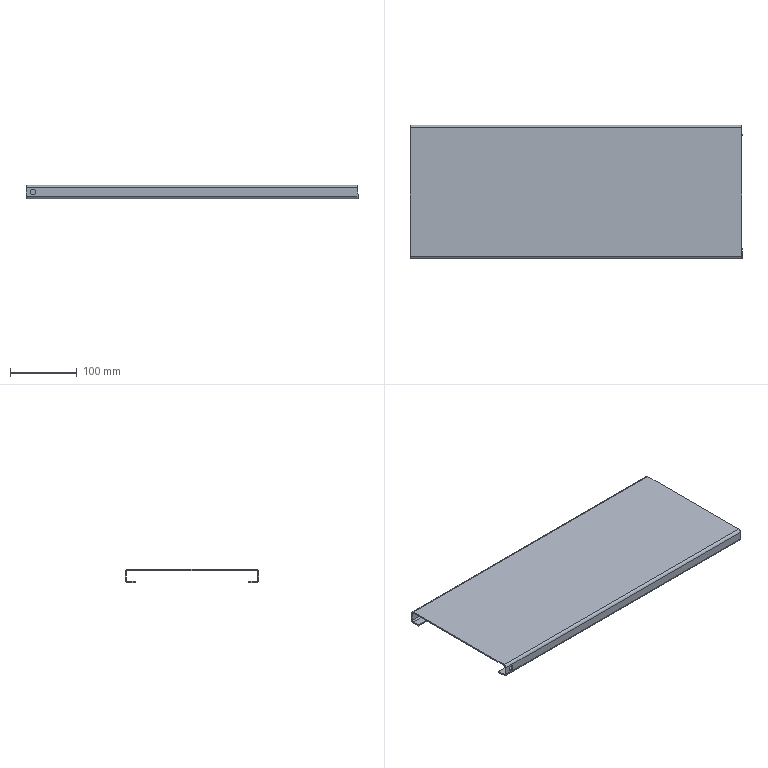Part | SolidWorks | features EdgeFlange 4, Extrusion 1, FlatPattern 1, ICE 1, SheetMetal 1, SolidToSheetMetal 1 | 1 solid | 40 faces | box 496 x 200 x 20 mm | volume 254694 mm3 | plane 30 | cylinder 10 | commonest cylinder face diameters 8 x6 4 x4
STEP:
#1=CARTESIAN_POINT('',(-237.5,-98.,-5.));
#2=VERTEX_POINT('',#1);
#3=CARTESIAN_POINT('',(-237.5,-98.,-13.));
#4=VERTEX_POINT('',#3);
#5=CARTESIAN_POINT('',(-237.5,-98.,-9.));
#6=DIRECTION('',(0.,-1.,0.));
#7=DIRECTION('',(0.,0.,-1.));
#8=AXIS2_PLACEMENT_3D('',#5,#6,#7);
#9=CIRCLE('',#8,4.);
#10=EDGE_CURVE('',#2,#4,#9,.T.);
#11=ORIENTED_EDGE('',*,*,#10,.F.);
#12=CARTESIAN_POINT('',(-237.5,-100.,-5.));
#13=VERTEX_POINT('',#12);
#14=CARTESIAN_POINT('',(-237.5,-98.,-5.));
#15=DIRECTION('',(0.,-1.,0.));
#16=VECTOR('',#15,1000.);
#17=LINE('',#14,#16);
#18=EDGE_CURVE('',#2,#13,#17,.T.);
#19=ORIENTED_EDGE('',*,*,#18,.T.);
#20=CARTESIAN_POINT('',(-237.5,-100.,-13.));
#21=VERTEX_POINT('',#20);
#22=CARTESIAN_POINT('',(-237.5,-100.,-9.));
#23=DIRECTION('',(0.,-1.,0.));
#24=DIRECTION('',(0.,0.,-1.));
#25=AXIS2_PLACEMENT_3D('',#22,#23,#24);
#26=CIRCLE('',#25,4.);
#27=EDGE_CURVE('',#13,#21,#26,.T.);
#28=ORIENTED_EDGE('',*,*,#27,.T.);
#29=CARTESIAN_POINT('',(-237.5,-98.,-13.));
#30=DIRECTION('',(0.,-1.,0.));
#31=VECTOR('',#30,1000.);
#32=LINE('',#29,#31);
#33=EDGE_CURVE('',#4,#21,#32,.T.);
#34=ORIENTED_EDGE('',*,*,#33,.F.);
#35=EDGE_LOOP('',(#11,#19,#28,#34));
#36=FACE_OUTER_BOUND('',#35,.T.);
#37=CARTESIAN_POINT('',(-237.5,-98.,-9.));
#38=DIRECTION('',(0.,-1.,0.));
#39=DIRECTION('',(0.,0.,-1.));
#40=AXIS2_PLACEMENT_3D('',#37,#38,#39);
#41=CYLINDRICAL_SURFACE('',#40,4.);
#42=ADVANCED_FACE('',(#36),#41,.F.);
#43=CARTESIAN_POINT('',(-248.,-98.,-15.));
#44=VERTEX_POINT('',#43);
#45=CARTESIAN_POINT('',(-248.,-98.,-3.));
#46=VERTEX_POINT('',#45);
#47=CARTESIAN_POINT('',(-248.,-98.,-1.));
#48=DIRECTION('',(0.,0.,1.));
#49=VECTOR('',#48,1000.);
#50=LINE('',#47,#49);
#51=EDGE_CURVE('',#44,#46,#50,.T.);
#52=ORIENTED_EDGE('',*,*,#51,.F.);
#53=CARTESIAN_POINT('',(-248.,-100.,-15.));
#54=VERTEX_POINT('',#53);
#55=CARTESIAN_POINT('',(-248.,-98.,-15.));
#56=DIRECTION('',(0.,-1.,0.));
#57=VECTOR('',#56,1000.);
#58=LINE('',#55,#57);
#59=EDGE_CURVE('',#44,#54,#58,.T.);
#60=ORIENTED_EDGE('',*,*,#59,.T.);
#61=CARTESIAN_POINT('',(-248.,-100.,-3.));
#62=VERTEX_POINT('',#61);
#63=CARTESIAN_POINT('',(-248.,-100.,-1.));
#64=DIRECTION('',(0.,0.,1.));
#65=VECTOR('',#64,1000.);
#66=LINE('',#63,#65);
#67=EDGE_CURVE('',#54,#62,#66,.T.);
#68=ORIENTED_EDGE('',*,*,#67,.T.);
#69=CARTESIAN_POINT('',(-248.,-98.,-3.));
#70=DIRECTION('',(0.,-1.,0.));
#71=VECTOR('',#70,1000.);
#72=LINE('',#69,#71);
#73=EDGE_CURVE('',#46,#62,#72,.T.);
#74=ORIENTED_EDGE('',*,*,#73,.F.);
#75=EDGE_LOOP('',(#52,#60,#68,#74));
#76=FACE_OUTER_BOUND('',#75,.T.);
#77=CARTESIAN_POINT('',(-248.,-100.,-1.));
#78=DIRECTION('',(-1.,0.,0.));
#79=DIRECTION('',(0.,0.,1.));
#80=AXIS2_PLACEMENT_3D('',#77,#78,#79);
#81=PLANE('',#80);
#82=ADVANCED_FACE('',(#76),#81,.T.);
#83=CARTESIAN_POINT('',(-237.5,-100.,-9.));
#84=DIRECTION('',(0.,-1.,0.));
#85=DIRECTION('',(0.,0.,-1.));
#86=AXIS2_PLACEMENT_3D('',#83,#84,#85);
#87=CIRCLE('',#86,4.);
#88=EDGE_CURVE('',#21,#13,#87,.T.);
#89=ORIENTED_EDGE('',*,*,#88,.F.);
#90=ORIENTED_EDGE('',*,*,#27,.F.);
#91=EDGE_LOOP('',(#89,#90));
#92=FACE_BOUND('',#91,.T.);
#93=ORIENTED_EDGE('',*,*,#67,.F.);
#94=CARTESIAN_POINT('',(248.,-100.,-15.));
#95=VERTEX_POINT('',#94);
#96=CARTESIAN_POINT('',(-248.,-100.,-15.));
#97=DIRECTION('',(1.,0.,0.));
#98=VECTOR('',#97,1000.);
#99=LINE('',#96,#98);
#100=EDGE_CURVE('',#54,#95,#99,.T.);
#101=ORIENTED_EDGE('',*,*,#100,.T.);
#102=CARTESIAN_POINT('',(248.,-100.,-3.));
#103=VERTEX_POINT('',#102);
#104=CARTESIAN_POINT('',(248.,-100.,-19.));
#105=DIRECTION('',(0.,0.,-1.));
#106=VECTOR('',#105,1000.);
#107=LINE('',#104,#106);
#108=EDGE_CURVE('',#103,#95,#107,.T.);
#109=ORIENTED_EDGE('',*,*,#108,.F.);
#110=CARTESIAN_POINT('',(-248.,-100.,-3.));
#111=DIRECTION('',(-1.,0.,0.));
#112=VECTOR('',#111,1000.);
#113=LINE('',#110,#112);
#114=EDGE_CURVE('',#103,#62,#113,.T.);
#115=ORIENTED_EDGE('',*,*,#114,.T.);
#116=EDGE_LOOP('',(#93,#101,#109,#115));
#117=FACE_OUTER_BOUND('',#116,.T.);
#118=CARTESIAN_POINT('',(-248.,-100.,-1.));
#119=DIRECTION('',(0.,-1.,0.));
#120=DIRECTION('',(0.,0.,-1.));
#121=AXIS2_PLACEMENT_3D('',#118,#119,#120);
#122=PLANE('',#121);
#123=ADVANCED_FACE('',(#92,#117),#122,.T.);
#124=CARTESIAN_POINT('',(-237.5,-98.,-9.));
#125=DIRECTION('',(0.,-1.,0.));
#126=DIRECTION('',(0.,0.,-1.));
#127=AXIS2_PLACEMENT_3D('',#124,#125,#126);
#128=CIRCLE('',#127,4.);
#129=EDGE_CURVE('',#4,#2,#128,.T.);
#130=ORIENTED_EDGE('',*,*,#129,.T.);
#131=ORIENTED_EDGE('',*,*,#10,.T.);
#132=EDGE_LOOP('',(#130,#131));
#133=FACE_BOUND('',#132,.T.);
#134=CARTESIAN_POINT('',(248.,-98.,-15.));
#135=VERTEX_POINT('',#134);
#136=CARTESIAN_POINT('',(-248.,-98.,-15.));
#137=DIRECTION('',(1.,0.,0.));
#138=VECTOR('',#137,1000.);
#139=LINE('',#136,#138);
#140=EDGE_CURVE('',#44,#135,#139,.T.);
#141=ORIENTED_EDGE('',*,*,#140,.F.);
#142=ORIENTED_EDGE('',*,*,#51,.T.);
#143=CARTESIAN_POINT('',(248.,-98.,-3.));
#144=VERTEX_POINT('',#143);
#145=CARTESIAN_POINT('',(248.,-98.,-3.));
#146=DIRECTION('',(-1.,0.,0.));
#147=VECTOR('',#146,1000.);
#148=LINE('',#145,#147);
#149=EDGE_CURVE('',#144,#46,#148,.T.);
#150=ORIENTED_EDGE('',*,*,#149,.F.);
#151=CARTESIAN_POINT('',(248.,-98.,-1.));
#152=DIRECTION('',(0.,0.,-1.));
#153=VECTOR('',#152,1000.);
#154=LINE('',#151,#153);
#155=EDGE_CURVE('',#144,#135,#154,.T.);
#156=ORIENTED_EDGE('',*,*,#155,.T.);
#157=EDGE_LOOP('',(#141,#142,#150,#156));
#158=FACE_OUTER_BOUND('',#157,.T.);
#159=CARTESIAN_POINT('',(-248.,-98.,-1.));
#160=DIRECTION('',(0.,-1.,0.));
#161=DIRECTION('',(0.,0.,-1.));
#162=AXIS2_PLACEMENT_3D('',#159,#160,#161);
#163=PLANE('',#162);
#164=ADVANCED_FACE('',(#133,#158),#163,.F.);
#165=CARTESIAN_POINT('',(-248.,96.,1.));
#166=VERTEX_POINT('',#165);
#167=CARTESIAN_POINT('',(-248.,-96.,1.));
#168=VERTEX_POINT('',#167);
#169=CARTESIAN_POINT('',(-248.,100.,1.));
#170=DIRECTION('',(0.,-1.,0.));
#171=VECTOR('',#170,1000.);
#172=LINE('',#169,#171);
#173=EDGE_CURVE('',#166,#168,#172,.T.);
#174=ORIENTED_EDGE('',*,*,#173,.T.);
#175=CARTESIAN_POINT('',(248.,-96.,1.));
#176=VERTEX_POINT('',#175);
#177=CARTESIAN_POINT('',(-248.,-96.,1.));
#178=DIRECTION('',(1.,0.,0.));
#179=VECTOR('',#178,1000.);
#180=LINE('',#177,#179);
#181=EDGE_CURVE('',#168,#176,#180,.T.);
#182=ORIENTED_EDGE('',*,*,#181,.T.);
#183=CARTESIAN_POINT('',(248.,96.,1.));
#184=VERTEX_POINT('',#183);
#185=CARTESIAN_POINT('',(248.,100.,1.));
#186=DIRECTION('',(0.,1.,0.));
#187=VECTOR('',#186,1000.);
#188=LINE('',#185,#187);
#189=EDGE_CURVE('',#176,#184,#188,.T.);
#190=ORIENTED_EDGE('',*,*,#189,.T.);
#191=CARTESIAN_POINT('',(248.,96.,1.));
#192=DIRECTION('',(-1.,0.,0.));
#193=VECTOR('',#192,1000.);
#194=LINE('',#191,#193);
#195=EDGE_CURVE('',#184,#166,#194,.T.);
#196=ORIENTED_EDGE('',*,*,#195,.T.);
#197=EDGE_LOOP('',(#174,#182,#190,#196));
#198=FACE_OUTER_BOUND('',#197,.T.);
#199=CARTESIAN_POINT('',(248.,-100.,1.));
#200=DIRECTION('',(0.,0.,1.));
#201=DIRECTION('',(1.,0.,0.));
#202=AXIS2_PLACEMENT_3D('',#199,#200,#201);
#203=PLANE('',#202);
#204=ADVANCED_FACE('',(#198),#203,.T.);
#205=CARTESIAN_POINT('',(-248.,-96.,-1.));
#206=VERTEX_POINT('',#205);
#207=CARTESIAN_POINT('',(248.,-96.,-1.));
#208=VERTEX_POINT('',#207);
#209=CARTESIAN_POINT('',(-248.,-96.,-1.));
#210=DIRECTION('',(1.,0.,0.));
#211=VECTOR('',#210,1000.);
#212=LINE('',#209,#211);
#213=EDGE_CURVE('',#206,#208,#212,.T.);
#214=ORIENTED_EDGE('',*,*,#213,.F.);
#215=CARTESIAN_POINT('',(-248.,96.,-1.));
#216=VERTEX_POINT('',#215);
#217=CARTESIAN_POINT('',(-248.,-100.,-1.));
#218=DIRECTION('',(0.,-1.,0.));
#219=VECTOR('',#218,1000.);
#220=LINE('',#217,#219);
#221=EDGE_CURVE('',#216,#206,#220,.T.);
#222=ORIENTED_EDGE('',*,*,#221,.F.);
#223=CARTESIAN_POINT('',(248.,96.,-1.));
#224=VERTEX_POINT('',#223);
#225=CARTESIAN_POINT('',(248.,96.,-1.));
#226=DIRECTION('',(-1.,0.,0.));
#227=VECTOR('',#226,1000.);
#228=LINE('',#225,#227);
#229=EDGE_CURVE('',#224,#216,#228,.T.);
#230=ORIENTED_EDGE('',*,*,#229,.F.);
#231=CARTESIAN_POINT('',(248.,-100.,-1.));
#232=DIRECTION('',(0.,1.,0.));
#233=VECTOR('',#232,1000.);
#234=LINE('',#231,#233);
#235=EDGE_CURVE('',#208,#224,#234,.T.);
#236=ORIENTED_EDGE('',*,*,#235,.F.);
#237=EDGE_LOOP('',(#214,#222,#230,#236));
#238=FACE_OUTER_BOUND('',#237,.T.);
#239=CARTESIAN_POINT('',(248.,-100.,-1.));
#240=DIRECTION('',(0.,0.,1.));
#241=DIRECTION('',(1.,0.,0.));
#242=AXIS2_PLACEMENT_3D('',#239,#240,#241);
#243=PLANE('',#242);
#244=ADVANCED_FACE('',(#238),#243,.F.);
#245=ORIENTED_EDGE('',*,*,#221,.T.);
#246=CARTESIAN_POINT('',(-248.,-96.,-1.));
#247=DIRECTION('',(0.,0.,1.));
#248=VECTOR('',#247,1000.);
#249=LINE('',#246,#248);
#250=EDGE_CURVE('',#206,#168,#249,.T.);
#251=ORIENTED_EDGE('',*,*,#250,.T.);
#252=ORIENTED_EDGE('',*,*,#173,.F.);
#253=CARTESIAN_POINT('',(-248.,96.,-1.));
#254=DIRECTION('',(0.,0.,1.));
#255=VECTOR('',#254,1000.);
#256=LINE('',#253,#255);
#257=EDGE_CURVE('',#216,#166,#256,.T.);
#258=ORIENTED_EDGE('',*,*,#257,.F.);
#259=EDGE_LOOP('',(#245,#251,#252,#258));
#260=FACE_OUTER_BOUND('',#259,.T.);
#261=CARTESIAN_POINT('',(-248.,100.,1.));
#262=DIRECTION('',(-1.,0.,0.));
#263=DIRECTION('',(0.,-1.,0.));
#264=AXIS2_PLACEMENT_3D('',#261,#262,#263);
#265=PLANE('',#264);
#266=ADVANCED_FACE('',(#260),#265,.T.);
#267=CARTESIAN_POINT('',(248.,98.,-15.));
#268=VERTEX_POINT('',#267);
#269=CARTESIAN_POINT('',(248.,98.,-3.));
#270=VERTEX_POINT('',#269);
#271=CARTESIAN_POINT('',(248.,98.,-1.));
#272=DIRECTION('',(0.,0.,1.));
#273=VECTOR('',#272,1000.);
#274=LINE('',#271,#273);
#275=EDGE_CURVE('',#268,#270,#274,.T.);
#276=ORIENTED_EDGE('',*,*,#275,.F.);
#277=CARTESIAN_POINT('',(248.,100.,-15.));
#278=VERTEX_POINT('',#277);
#279=CARTESIAN_POINT('',(248.,98.,-15.));
#280=DIRECTION('',(0.,1.,0.));
#281=VECTOR('',#280,1000.);
#282=LINE('',#279,#281);
#283=EDGE_CURVE('',#268,#278,#282,.T.);
#284=ORIENTED_EDGE('',*,*,#283,.T.);
#285=CARTESIAN_POINT('',(248.,100.,-3.));
#286=VERTEX_POINT('',#285);
#287=CARTESIAN_POINT('',(248.,100.,-1.));
#288=DIRECTION('',(0.,0.,1.));
#289=VECTOR('',#288,1000.);
#290=LINE('',#287,#289);
#291=EDGE_CURVE('',#278,#286,#290,.T.);
#292=ORIENTED_EDGE('',*,*,#291,.T.);
#293=CARTESIAN_POINT('',(248.,98.,-3.));
#294=DIRECTION('',(0.,1.,0.));
#295=VECTOR('',#294,1000.);
#296=LINE('',#293,#295);
#297=EDGE_CURVE('',#270,#286,#296,.T.);
#298=ORIENTED_EDGE('',*,*,#297,.F.);
#299=EDGE_LOOP('',(#276,#284,#292,#298));
#300=FACE_OUTER_BOUND('',#299,.T.);
#301=CARTESIAN_POINT('',(248.,100.,-1.));
#302=DIRECTION('',(1.,0.,0.));
#303=DIRECTION('',(0.,0.,-1.));
#304=AXIS2_PLACEMENT_3D('',#301,#302,#303);
#305=PLANE('',#304);
#306=ADVANCED_FACE('',(#300),#305,.T.);
#307=ORIENTED_EDGE('',*,*,#291,.F.);
#308=CARTESIAN_POINT('',(-248.,100.,-15.));
#309=VERTEX_POINT('',#308);
#310=CARTESIAN_POINT('',(248.,100.,-15.));
#311=DIRECTION('',(-1.,0.,0.));
#312=VECTOR('',#311,1000.);
#313=LINE('',#310,#312);
#314=EDGE_CURVE('',#278,#309,#313,.T.);
#315=ORIENTED_EDGE('',*,*,#314,.T.);
#316=CARTESIAN_POINT('',(-248.,100.,-3.));
#317=VERTEX_POINT('',#316);
#318=CARTESIAN_POINT('',(-248.,100.,-19.));
#319=DIRECTION('',(0.,0.,-1.));
#320=VECTOR('',#319,1000.);
#321=LINE('',#318,#320);
#322=EDGE_CURVE('',#317,#309,#321,.T.);
#323=ORIENTED_EDGE('',*,*,#322,.F.);
#324=CARTESIAN_POINT('',(248.,100.,-3.));
#325=DIRECTION('',(1.,0.,0.));
#326=VECTOR('',#325,1000.);
#327=LINE('',#324,#326);
#328=EDGE_CURVE('',#317,#286,#327,.T.);
#329=ORIENTED_EDGE('',*,*,#328,.T.);
#330=EDGE_LOOP('',(#307,#315,#323,#329));
#331=FACE_OUTER_BOUND('',#330,.T.);
#332=CARTESIAN_POINT('',(248.,100.,-1.));
#333=DIRECTION('',(0.,1.,0.));
#334=DIRECTION('',(0.,0.,1.));
#335=AXIS2_PLACEMENT_3D('',#332,#333,#334);
#336=PLANE('',#335);
#337=ADVANCED_FACE('',(#331),#336,.T.);
#338=CARTESIAN_POINT('',(-248.,98.,-15.));
#339=VERTEX_POINT('',#338);
#340=CARTESIAN_POINT('',(248.,98.,-15.));
#341=DIRECTION('',(-1.,0.,0.));
#342=VECTOR('',#341,1000.);
#343=LINE('',#340,#342);
#344=EDGE_CURVE('',#268,#339,#343,.T.);
#345=ORIENTED_EDGE('',*,*,#344,.F.);
#346=ORIENTED_EDGE('',*,*,#275,.T.);
#347=CARTESIAN_POINT('',(-248.,98.,-3.));
#348=VERTEX_POINT('',#347);
#349=CARTESIAN_POINT('',(-248.,98.,-3.));
#350=DIRECTION('',(1.,0.,0.));
#351=VECTOR('',#350,1000.);
#352=LINE('',#349,#351);
#353=EDGE_CURVE('',#348,#270,#352,.T.);
#354=ORIENTED_EDGE('',*,*,#353,.F.);
#355=CARTESIAN_POINT('',(-248.,98.,-1.));
#356=DIRECTION('',(0.,0.,-1.));
#357=VECTOR('',#356,1000.);
#358=LINE('',#355,#357);
#359=EDGE_CURVE('',#348,#339,#358,.T.);
#360=ORIENTED_EDGE('',*,*,#359,.T.);
#361=EDGE_LOOP('',(#345,#346,#354,#360));
#362=FACE_OUTER_BOUND('',#361,.T.);
#363=CARTESIAN_POINT('',(248.,98.,-1.));
#364=DIRECTION('',(0.,1.,0.));
#365=DIRECTION('',(0.,0.,1.));
#366=AXIS2_PLACEMENT_3D('',#363,#364,#365);
#367=PLANE('',#366);
#368=ADVANCED_FACE('',(#362),#367,.F.);
#369=CARTESIAN_POINT('',(248.,-96.,-1.));
#370=DIRECTION('',(0.,0.,1.));
#371=VECTOR('',#370,1000.);
#372=LINE('',#369,#371);
#373=EDGE_CURVE('',#208,#176,#372,.T.);
#374=ORIENTED_EDGE('',*,*,#373,.F.);
#375=ORIENTED_EDGE('',*,*,#235,.T.);
#376=CARTESIAN_POINT('',(248.,96.,-1.));
#377=DIRECTION('',(0.,0.,1.));
#378=VECTOR('',#377,1000.);
#379=LINE('',#376,#378);
#380=EDGE_CURVE('',#224,#184,#379,.T.);
#381=ORIENTED_EDGE('',*,*,#380,.T.);
#382=ORIENTED_EDGE('',*,*,#189,.F.);
#383=EDGE_LOOP('',(#374,#375,#381,#382));
#384=FACE_OUTER_BOUND('',#383,.T.);
#385=CARTESIAN_POINT('',(248.,100.,1.));
#386=DIRECTION('',(1.,0.,0.));
#387=DIRECTION('',(0.,1.,0.));
#388=AXIS2_PLACEMENT_3D('',#385,#386,#387);
#389=PLANE('',#388);
#390=ADVANCED_FACE('',(#384),#389,.T.);
#391=CARTESIAN_POINT('',(-248.,100.,-3.));
#392=DIRECTION('',(0.,1.,0.));
#393=VECTOR('',#392,1000.);
#394=LINE('',#391,#393);
#395=EDGE_CURVE('',#348,#317,#394,.T.);
#396=ORIENTED_EDGE('',*,*,#395,.F.);
#397=CARTESIAN_POINT('',(-248.,96.,-3.));
#398=DIRECTION('',(-1.,0.,0.));
#399=DIRECTION('',(0.,0.,-1.));
#400=AXIS2_PLACEMENT_3D('',#397,#398,#399);
#401=CIRCLE('',#400,2.);
#402=EDGE_CURVE('',#216,#348,#401,.T.);
#403=ORIENTED_EDGE('',*,*,#402,.F.);
#404=ORIENTED_EDGE('',*,*,#257,.T.);
#405=CARTESIAN_POINT('',(-248.,96.,-3.));
#406=DIRECTION('',(-1.,0.,0.));
#407=DIRECTION('',(0.,0.,-1.));
#408=AXIS2_PLACEMENT_3D('',#405,#406,#407);
#409=CIRCLE('',#408,4.);
#410=EDGE_CURVE('',#166,#317,#409,.T.);
#411=ORIENTED_EDGE('',*,*,#410,.T.);
#412=EDGE_LOOP('',(#396,#403,#404,#411));
#413=FACE_OUTER_BOUND('',#412,.T.);
#414=CARTESIAN_POINT('',(-248.,96.,-3.));
#415=DIRECTION('',(-1.,0.,0.));
#416=DIRECTION('',(0.,0.,1.));
#417=AXIS2_PLACEMENT_3D('',#414,#415,#416);
#418=PLANE('',#417);
#419=ADVANCED_FACE('',(#413),#418,.T.);
#420=ORIENTED_EDGE('',*,*,#195,.F.);
#421=CARTESIAN_POINT('',(248.,96.,-3.));
#422=DIRECTION('',(1.,0.,0.));
#423=DIRECTION('',(0.,0.,-1.));
#424=AXIS2_PLACEMENT_3D('',#421,#422,#423);
#425=CIRCLE('',#424,4.);
#426=EDGE_CURVE('',#286,#184,#425,.T.);
#427=ORIENTED_EDGE('',*,*,#426,.F.);
#428=ORIENTED_EDGE('',*,*,#328,.F.);
#429=ORIENTED_EDGE('',*,*,#410,.F.);
#430=EDGE_LOOP('',(#420,#427,#428,#429));
#431=FACE_OUTER_BOUND('',#430,.T.);
#432=CARTESIAN_POINT('',(248.,96.,-3.));
#433=DIRECTION('',(1.,0.,0.));
#434=DIRECTION('',(0.,1.,0.));
#435=AXIS2_PLACEMENT_3D('',#432,#433,#434);
#436=CYLINDRICAL_SURFACE('',#435,4.);
#437=ADVANCED_FACE('',(#431),#436,.T.);
#438=CARTESIAN_POINT('',(248.,96.,-3.));
#439=DIRECTION('',(1.,0.,0.));
#440=DIRECTION('',(0.,0.,-1.));
#441=AXIS2_PLACEMENT_3D('',#438,#439,#440);
#442=CIRCLE('',#441,2.);
#443=EDGE_CURVE('',#270,#224,#442,.T.);
#444=ORIENTED_EDGE('',*,*,#443,.F.);
#445=ORIENTED_EDGE('',*,*,#297,.T.);
#446=ORIENTED_EDGE('',*,*,#426,.T.);
#447=ORIENTED_EDGE('',*,*,#380,.F.);
#448=EDGE_LOOP('',(#444,#445,#446,#447));
#449=FACE_OUTER_BOUND('',#448,.T.);
#450=CARTESIAN_POINT('',(248.,96.,-3.));
#451=DIRECTION('',(-1.,0.,0.));
#452=DIRECTION('',(0.,0.,1.));
#453=AXIS2_PLACEMENT_3D('',#450,#451,#452);
#454=PLANE('',#453);
#455=ADVANCED_FACE('',(#449),#454,.F.);
#456=ORIENTED_EDGE('',*,*,#229,.T.);
#457=ORIENTED_EDGE('',*,*,#402,.T.);
#458=ORIENTED_EDGE('',*,*,#353,.T.);
#459=ORIENTED_EDGE('',*,*,#443,.T.);
#460=EDGE_LOOP('',(#456,#457,#458,#459));
#461=FACE_OUTER_BOUND('',#460,.T.);
#462=CARTESIAN_POINT('',(248.,96.,-3.));
#463=DIRECTION('',(1.,0.,0.));
#464=DIRECTION('',(0.,1.,0.));
#465=AXIS2_PLACEMENT_3D('',#462,#463,#464);
#466=CYLINDRICAL_SURFACE('',#465,2.);
#467=ADVANCED_FACE('',(#461),#466,.F.);
#468=CARTESIAN_POINT('',(-248.,98.,-15.));
#469=DIRECTION('',(0.,1.,0.));
#470=VECTOR('',#469,1000.);
#471=LINE('',#468,#470);
#472=EDGE_CURVE('',#339,#309,#471,.T.);
#473=ORIENTED_EDGE('',*,*,#472,.F.);
#474=ORIENTED_EDGE('',*,*,#359,.F.);
#475=ORIENTED_EDGE('',*,*,#395,.T.);
#476=ORIENTED_EDGE('',*,*,#322,.T.);
#477=EDGE_LOOP('',(#473,#474,#475,#476));
#478=FACE_OUTER_BOUND('',#477,.T.);
#479=CARTESIAN_POINT('',(-248.,100.,-19.));
#480=DIRECTION('',(-1.,0.,0.));
#481=DIRECTION('',(0.,0.,1.));
#482=AXIS2_PLACEMENT_3D('',#479,#480,#481);
#483=PLANE('',#482);
#484=ADVANCED_FACE('',(#478),#483,.T.);
#485=CARTESIAN_POINT('',(-248.,96.,-17.));
#486=VERTEX_POINT('',#485);
#487=CARTESIAN_POINT('',(-248.,96.,-19.));
#488=VERTEX_POINT('',#487);
#489=CARTESIAN_POINT('',(-248.,96.,-19.));
#490=DIRECTION('',(0.,0.,-1.));
#491=VECTOR('',#490,1000.);
#492=LINE('',#489,#491);
#493=EDGE_CURVE('',#486,#488,#492,.T.);
#494=ORIENTED_EDGE('',*,*,#493,.F.);
#495=CARTESIAN_POINT('',(-248.,96.,-15.));
#496=DIRECTION('',(-1.,0.,0.));
#497=DIRECTION('',(0.,0.,-1.));
#498=AXIS2_PLACEMENT_3D('',#495,#496,#497);
#499=CIRCLE('',#498,2.);
#500=EDGE_CURVE('',#339,#486,#499,.T.);
#501=ORIENTED_EDGE('',*,*,#500,.F.);
#502=ORIENTED_EDGE('',*,*,#472,.T.);
#503=CARTESIAN_POINT('',(-248.,96.,-15.));
#504=DIRECTION('',(-1.,0.,0.));
#505=DIRECTION('',(0.,0.,-1.));
#506=AXIS2_PLACEMENT_3D('',#503,#504,#505);
#507=CIRCLE('',#506,4.);
#508=EDGE_CURVE('',#309,#488,#507,.T.);
#509=ORIENTED_EDGE('',*,*,#508,.T.);
#510=EDGE_LOOP('',(#494,#501,#502,#509));
#511=FACE_OUTER_BOUND('',#510,.T.);
#512=CARTESIAN_POINT('',(-248.,96.,-15.));
#513=DIRECTION('',(-1.,0.,0.));
#514=DIRECTION('',(0.,0.,1.));
#515=AXIS2_PLACEMENT_3D('',#512,#513,#514);
#516=PLANE('',#515);
#517=ADVANCED_FACE('',(#511),#516,.T.);
#518=ORIENTED_EDGE('',*,*,#314,.F.);
#519=CARTESIAN_POINT('',(248.,96.,-19.));
#520=VERTEX_POINT('',#519);
#521=CARTESIAN_POINT('',(248.,96.,-15.));
#522=DIRECTION('',(1.,0.,0.));
#523=DIRECTION('',(0.,0.,-1.));
#524=AXIS2_PLACEMENT_3D('',#521,#522,#523);
#525=CIRCLE('',#524,4.);
#526=EDGE_CURVE('',#520,#278,#525,.T.);
#527=ORIENTED_EDGE('',*,*,#526,.F.);
#528=CARTESIAN_POINT('',(248.,96.,-19.));
#529=DIRECTION('',(1.,0.,0.));
#530=VECTOR('',#529,1000.);
#531=LINE('',#528,#530);
#532=EDGE_CURVE('',#488,#520,#531,.T.);
#533=ORIENTED_EDGE('',*,*,#532,.F.);
#534=ORIENTED_EDGE('',*,*,#508,.F.);
#535=EDGE_LOOP('',(#518,#527,#533,#534));
#536=FACE_OUTER_BOUND('',#535,.T.);
#537=CARTESIAN_POINT('',(248.,96.,-15.));
#538=DIRECTION('',(1.,0.,0.));
#539=DIRECTION('',(0.,0.,-1.));
#540=AXIS2_PLACEMENT_3D('',#537,#538,#539);
#541=CYLINDRICAL_SURFACE('',#540,4.);
#542=ADVANCED_FACE('',(#536),#541,.T.);
#543=CARTESIAN_POINT('',(248.,96.,-17.));
#544=VERTEX_POINT('',#543);
#545=CARTESIAN_POINT('',(248.,96.,-15.));
#546=DIRECTION('',(1.,0.,0.));
#547=DIRECTION('',(0.,0.,-1.));
#548=AXIS2_PLACEMENT_3D('',#545,#546,#547);
#549=CIRCLE('',#548,2.);
#550=EDGE_CURVE('',#544,#268,#549,.T.);
#551=ORIENTED_EDGE('',*,*,#550,.F.);
#552=CARTESIAN_POINT('',(248.,96.,-17.));
#553=DIRECTION('',(0.,0.,-1.));
#554=VECTOR('',#553,1000.);
#555=LINE('',#552,#554);
#556=EDGE_CURVE('',#544,#520,#555,.T.);
#557=ORIENTED_EDGE('',*,*,#556,.T.);
#558=ORIENTED_EDGE('',*,*,#526,.T.);
#559=ORIENTED_EDGE('',*,*,#283,.F.);
#560=EDGE_LOOP('',(#551,#557,#558,#559));
#561=FACE_OUTER_BOUND('',#560,.T.);
#562=CARTESIAN_POINT('',(248.,96.,-15.));
#563=DIRECTION('',(-1.,0.,0.));
#564=DIRECTION('',(0.,0.,1.));
#565=AXIS2_PLACEMENT_3D('',#562,#563,#564);
#566=PLANE('',#565);
#567=ADVANCED_FACE('',(#561),#566,.F.);
#568=ORIENTED_EDGE('',*,*,#344,.T.);
#569=ORIENTED_EDGE('',*,*,#500,.T.);
#570=CARTESIAN_POINT('',(-248.,96.,-17.));
#571=DIRECTION('',(1.,0.,0.));
#572=VECTOR('',#571,1000.);
#573=LINE('',#570,#572);
#574=EDGE_CURVE('',#486,#544,#573,.T.);
#575=ORIENTED_EDGE('',*,*,#574,.T.);
#576=ORIENTED_EDGE('',*,*,#550,.T.);
#577=EDGE_LOOP('',(#568,#569,#575,#576));
#578=FACE_OUTER_BOUND('',#577,.T.);
#579=CARTESIAN_POINT('',(248.,96.,-15.));
#580=DIRECTION('',(1.,0.,0.));
#581=DIRECTION('',(0.,0.,-1.));
#582=AXIS2_PLACEMENT_3D('',#579,#580,#581);
#583=CYLINDRICAL_SURFACE('',#582,2.);
#584=ADVANCED_FACE('',(#578),#583,.F.);
#585=CARTESIAN_POINT('',(248.,85.,-19.));
#586=VERTEX_POINT('',#585);
#587=CARTESIAN_POINT('',(248.,98.,-19.));
#588=DIRECTION('',(0.,1.,0.));
#589=VECTOR('',#588,1000.);
#590=LINE('',#587,#589);
#591=EDGE_CURVE('',#586,#520,#590,.T.);
#592=ORIENTED_EDGE('',*,*,#591,.T.);
#593=ORIENTED_EDGE('',*,*,#556,.F.);
#594=CARTESIAN_POINT('',(248.,85.,-17.));
#595=VERTEX_POINT('',#594);
#596=CARTESIAN_POINT('',(248.,98.,-17.));
#597=DIRECTION('',(0.,1.,0.));
#598=VECTOR('',#597,1000.);
#599=LINE('',#596,#598);
#600=EDGE_CURVE('',#595,#544,#599,.T.);
#601=ORIENTED_EDGE('',*,*,#600,.F.);
#602=CARTESIAN_POINT('',(248.,85.,-19.));
#603=DIRECTION('',(0.,0.,1.));
#604=VECTOR('',#603,1000.);
#605=LINE('',#602,#604);
#606=EDGE_CURVE('',#586,#595,#605,.T.);
#607=ORIENTED_EDGE('',*,*,#606,.F.);
#608=EDGE_LOOP('',(#592,#593,#601,#607));
#609=FACE_OUTER_BOUND('',#608,.T.);
#610=CARTESIAN_POINT('',(248.,98.,-19.));
#611=DIRECTION('',(1.,0.,0.));
#612=DIRECTION('',(0.,0.,-1.));
#613=AXIS2_PLACEMENT_3D('',#610,#611,#612);
#614=PLANE('',#613);
#615=ADVANCED_FACE('',(#609),#614,.T.);
#616=CARTESIAN_POINT('',(-248.,85.,-17.));
#617=VERTEX_POINT('',#616);
#618=CARTESIAN_POINT('',(-248.,98.,-17.));
#619=DIRECTION('',(0.,-1.,0.));
#620=VECTOR('',#619,1000.);
#621=LINE('',#618,#620);
#622=EDGE_CURVE('',#486,#617,#621,.T.);
#623=ORIENTED_EDGE('',*,*,#622,.F.);
#624=ORIENTED_EDGE('',*,*,#493,.T.);
#625=CARTESIAN_POINT('',(-248.,85.,-19.));
#626=VERTEX_POINT('',#625);
#627=CARTESIAN_POINT('',(-248.,85.,-19.));
#628=DIRECTION('',(0.,-1.,0.));
#629=VECTOR('',#628,1000.);
#630=LINE('',#627,#629);
#631=EDGE_CURVE('',#488,#626,#630,.T.);
#632=ORIENTED_EDGE('',*,*,#631,.T.);
#633=CARTESIAN_POINT('',(-248.,85.,-19.));
#634=DIRECTION('',(0.,0.,1.));
#635=VECTOR('',#634,1000.);
#636=LINE('',#633,#635);
#637=EDGE_CURVE('',#626,#617,#636,.T.);
#638=ORIENTED_EDGE('',*,*,#637,.T.);
#639=EDGE_LOOP('',(#623,#624,#632,#638));
#640=FACE_OUTER_BOUND('',#639,.T.);
#641=CARTESIAN_POINT('',(-248.,85.,-19.));
#642=DIRECTION('',(-1.,0.,0.));
#643=DIRECTION('',(0.,-1.,0.));
#644=AXIS2_PLACEMENT_3D('',#641,#642,#643);
#645=PLANE('',#644);
#646=ADVANCED_FACE('',(#640),#645,.T.);
#647=ORIENTED_EDGE('',*,*,#631,.F.);
#648=ORIENTED_EDGE('',*,*,#532,.T.);
#649=ORIENTED_EDGE('',*,*,#591,.F.);
#650=CARTESIAN_POINT('',(248.,85.,-19.));
#651=DIRECTION('',(1.,0.,0.));
#652=VECTOR('',#651,1000.);
#653=LINE('',#650,#652);
#654=EDGE_CURVE('',#626,#586,#653,.T.);
#655=ORIENTED_EDGE('',*,*,#654,.F.);
#656=EDGE_LOOP('',(#647,#648,#649,#655));
#657=FACE_OUTER_BOUND('',#656,.T.);
#658=CARTESIAN_POINT('',(248.,98.,-19.));
#659=DIRECTION('',(0.,0.,-1.));
#660=DIRECTION('',(0.,1.,0.));
#661=AXIS2_PLACEMENT_3D('',#658,#659,#660);
#662=PLANE('',#661);
#663=ADVANCED_FACE('',(#657),#662,.T.);
#664=ORIENTED_EDGE('',*,*,#574,.F.);
#665=ORIENTED_EDGE('',*,*,#622,.T.);
#666=CARTESIAN_POINT('',(248.,85.,-17.));
#667=DIRECTION('',(1.,0.,0.));
#668=VECTOR('',#667,1000.);
#669=LINE('',#666,#668);
#670=EDGE_CURVE('',#617,#595,#669,.T.);
#671=ORIENTED_EDGE('',*,*,#670,.T.);
#672=ORIENTED_EDGE('',*,*,#600,.T.);
#673=EDGE_LOOP('',(#664,#665,#671,#672));
#674=FACE_OUTER_BOUND('',#673,.T.);
#675=CARTESIAN_POINT('',(248.,98.,-17.));
#676=DIRECTION('',(0.,0.,-1.));
#677=DIRECTION('',(0.,1.,0.));
#678=AXIS2_PLACEMENT_3D('',#675,#676,#677);
#679=PLANE('',#678);
#680=ADVANCED_FACE('',(#674),#679,.F.);
#681=ORIENTED_EDGE('',*,*,#670,.F.);
#682=ORIENTED_EDGE('',*,*,#637,.F.);
#683=ORIENTED_EDGE('',*,*,#654,.T.);
#684=ORIENTED_EDGE('',*,*,#606,.T.);
#685=EDGE_LOOP('',(#681,#682,#683,#684));
#686=FACE_OUTER_BOUND('',#685,.T.);
#687=CARTESIAN_POINT('',(248.,85.,-19.));
#688=DIRECTION('',(0.,-1.,0.));
#689=DIRECTION('',(0.,0.,-1.));
#690=AXIS2_PLACEMENT_3D('',#687,#688,#689);
#691=PLANE('',#690);
#692=ADVANCED_FACE('',(#686),#691,.T.);
#693=CARTESIAN_POINT('',(248.,-100.,-3.));
#694=DIRECTION('',(0.,-1.,0.));
#695=VECTOR('',#694,1000.);
#696=LINE('',#693,#695);
#697=EDGE_CURVE('',#144,#103,#696,.T.);
#698=ORIENTED_EDGE('',*,*,#697,.F.);
#699=CARTESIAN_POINT('',(248.,-96.,-3.));
#700=DIRECTION('',(1.,0.,0.));
#701=DIRECTION('',(0.,0.,1.));
#702=AXIS2_PLACEMENT_3D('',#699,#700,#701);
#703=CIRCLE('',#702,2.);
#704=EDGE_CURVE('',#208,#144,#703,.T.);
#705=ORIENTED_EDGE('',*,*,#704,.F.);
#706=ORIENTED_EDGE('',*,*,#373,.T.);
#707=CARTESIAN_POINT('',(248.,-96.,-3.));
#708=DIRECTION('',(1.,0.,0.));
#709=DIRECTION('',(0.,0.,1.));
#710=AXIS2_PLACEMENT_3D('',#707,#708,#709);
#711=CIRCLE('',#710,4.);
#712=EDGE_CURVE('',#176,#103,#711,.T.);
#713=ORIENTED_EDGE('',*,*,#712,.T.);
#714=EDGE_LOOP('',(#698,#705,#706,#713));
#715=FACE_OUTER_BOUND('',#714,.T.);
#716=CARTESIAN_POINT('',(248.,-96.,-3.));
#717=DIRECTION('',(1.,0.,0.));
#718=DIRECTION('',(0.,0.,-1.));
#719=AXIS2_PLACEMENT_3D('',#716,#717,#718);
#720=PLANE('',#719);
#721=ADVANCED_FACE('',(#715),#720,.T.);
#722=ORIENTED_EDGE('',*,*,#181,.F.);
#723=CARTESIAN_POINT('',(-248.,-96.,-3.));
#724=DIRECTION('',(-1.,0.,0.));
#725=DIRECTION('',(0.,0.,1.));
#726=AXIS2_PLACEMENT_3D('',#723,#724,#725);
#727=CIRCLE('',#726,4.);
#728=EDGE_CURVE('',#62,#168,#727,.T.);
#729=ORIENTED_EDGE('',*,*,#728,.F.);
#730=ORIENTED_EDGE('',*,*,#114,.F.);
#731=ORIENTED_EDGE('',*,*,#712,.F.);
#732=EDGE_LOOP('',(#722,#729,#730,#731));
#733=FACE_OUTER_BOUND('',#732,.T.);
#734=CARTESIAN_POINT('',(-248.,-96.,-3.));
#735=DIRECTION('',(-1.,0.,0.));
#736=DIRECTION('',(0.,-1.,0.));
#737=AXIS2_PLACEMENT_3D('',#734,#735,#736);
#738=CYLINDRICAL_SURFACE('',#737,4.);
#739=ADVANCED_FACE('',(#733),#738,.T.);
#740=CARTESIAN_POINT('',(-248.,-96.,-3.));
#741=DIRECTION('',(-1.,0.,0.));
#742=DIRECTION('',(0.,0.,1.));
#743=AXIS2_PLACEMENT_3D('',#740,#741,#742);
#744=CIRCLE('',#743,2.);
#745=EDGE_CURVE('',#46,#206,#744,.T.);
#746=ORIENTED_EDGE('',*,*,#745,.F.);
#747=ORIENTED_EDGE('',*,*,#73,.T.);
#748=ORIENTED_EDGE('',*,*,#728,.T.);
#749=ORIENTED_EDGE('',*,*,#250,.F.);
#750=EDGE_LOOP('',(#746,#747,#748,#749));
#751=FACE_OUTER_BOUND('',#750,.T.);
#752=CARTESIAN_POINT('',(-248.,-96.,-3.));
#753=DIRECTION('',(1.,0.,0.));
#754=DIRECTION('',(0.,0.,-1.));
#755=AXIS2_PLACEMENT_3D('',#752,#753,#754);
#756=PLANE('',#755);
#757=ADVANCED_FACE('',(#751),#756,.F.);
#758=ORIENTED_EDGE('',*,*,#213,.T.);
#759=ORIENTED_EDGE('',*,*,#704,.T.);
#760=ORIENTED_EDGE('',*,*,#149,.T.);
#761=ORIENTED_EDGE('',*,*,#745,.T.);
#762=EDGE_LOOP('',(#758,#759,#760,#761));
#763=FACE_OUTER_BOUND('',#762,.T.);
#764=CARTESIAN_POINT('',(-248.,-96.,-3.));
#765=DIRECTION('',(-1.,0.,0.));
#766=DIRECTION('',(0.,-1.,0.));
#767=AXIS2_PLACEMENT_3D('',#764,#765,#766);
#768=CYLINDRICAL_SURFACE('',#767,2.);
#769=ADVANCED_FACE('',(#763),#768,.F.);
#770=CARTESIAN_POINT('',(248.,-98.,-15.));
#771=DIRECTION('',(0.,-1.,0.));
#772=VECTOR('',#771,1000.);
#773=LINE('',#770,#772);
#774=EDGE_CURVE('',#135,#95,#773,.T.);
#775=ORIENTED_EDGE('',*,*,#774,.F.);
#776=ORIENTED_EDGE('',*,*,#155,.F.);
#777=ORIENTED_EDGE('',*,*,#697,.T.);
#778=ORIENTED_EDGE('',*,*,#108,.T.);
#779=EDGE_LOOP('',(#775,#776,#777,#778));
#780=FACE_OUTER_BOUND('',#779,.T.);
#781=CARTESIAN_POINT('',(248.,-100.,-19.));
#782=DIRECTION('',(1.,0.,0.));
#783=DIRECTION('',(0.,0.,-1.));
#784=AXIS2_PLACEMENT_3D('',#781,#782,#783);
#785=PLANE('',#784);
#786=ADVANCED_FACE('',(#780),#785,.T.);
#787=CARTESIAN_POINT('',(248.,-96.,-17.));
#788=VERTEX_POINT('',#787);
#789=CARTESIAN_POINT('',(248.,-96.,-19.));
#790=VERTEX_POINT('',#789);
#791=CARTESIAN_POINT('',(248.,-96.,-19.));
#792=DIRECTION('',(0.,0.,-1.));
#793=VECTOR('',#792,1000.);
#794=LINE('',#791,#793);
#795=EDGE_CURVE('',#788,#790,#794,.T.);
#796=ORIENTED_EDGE('',*,*,#795,.F.);
#797=CARTESIAN_POINT('',(248.,-96.,-15.));
#798=DIRECTION('',(1.,0.,0.));
#799=DIRECTION('',(0.,0.,1.));
#800=AXIS2_PLACEMENT_3D('',#797,#798,#799);
#801=CIRCLE('',#800,2.);
#802=EDGE_CURVE('',#135,#788,#801,.T.);
#803=ORIENTED_EDGE('',*,*,#802,.F.);
#804=ORIENTED_EDGE('',*,*,#774,.T.);
#805=CARTESIAN_POINT('',(248.,-96.,-15.));
#806=DIRECTION('',(1.,0.,0.));
#807=DIRECTION('',(0.,0.,1.));
#808=AXIS2_PLACEMENT_3D('',#805,#806,#807);
#809=CIRCLE('',#808,4.);
#810=EDGE_CURVE('',#95,#790,#809,.T.);
#811=ORIENTED_EDGE('',*,*,#810,.T.);
#812=EDGE_LOOP('',(#796,#803,#804,#811));
#813=FACE_OUTER_BOUND('',#812,.T.);
#814=CARTESIAN_POINT('',(248.,-96.,-15.));
#815=DIRECTION('',(1.,0.,0.));
#816=DIRECTION('',(0.,0.,-1.));
#817=AXIS2_PLACEMENT_3D('',#814,#815,#816);
#818=PLANE('',#817);
#819=ADVANCED_FACE('',(#813),#818,.T.);
#820=ORIENTED_EDGE('',*,*,#100,.F.);
#821=CARTESIAN_POINT('',(-248.,-96.,-19.));
#822=VERTEX_POINT('',#821);
#823=CARTESIAN_POINT('',(-248.,-96.,-15.));
#824=DIRECTION('',(-1.,0.,0.));
#825=DIRECTION('',(0.,0.,1.));
#826=AXIS2_PLACEMENT_3D('',#823,#824,#825);
#827=CIRCLE('',#826,4.);
#828=EDGE_CURVE('',#822,#54,#827,.T.);
#829=ORIENTED_EDGE('',*,*,#828,.F.);
#830=CARTESIAN_POINT('',(-248.,-96.,-19.));
#831=DIRECTION('',(-1.,0.,0.));
#832=VECTOR('',#831,1000.);
#833=LINE('',#830,#832);
#834=EDGE_CURVE('',#790,#822,#833,.T.);
#835=ORIENTED_EDGE('',*,*,#834,.F.);
#836=ORIENTED_EDGE('',*,*,#810,.F.);
#837=EDGE_LOOP('',(#820,#829,#835,#836));
#838=FACE_OUTER_BOUND('',#837,.T.);
#839=CARTESIAN_POINT('',(-248.,-96.,-15.));
#840=DIRECTION('',(-1.,0.,0.));
#841=DIRECTION('',(0.,0.,-1.));
#842=AXIS2_PLACEMENT_3D('',#839,#840,#841);
#843=CYLINDRICAL_SURFACE('',#842,4.);
#844=ADVANCED_FACE('',(#838),#843,.T.);
#845=CARTESIAN_POINT('',(-248.,-96.,-17.));
#846=VERTEX_POINT('',#845);
#847=CARTESIAN_POINT('',(-248.,-96.,-15.));
#848=DIRECTION('',(-1.,0.,0.));
#849=DIRECTION('',(0.,0.,1.));
#850=AXIS2_PLACEMENT_3D('',#847,#848,#849);
#851=CIRCLE('',#850,2.);
#852=EDGE_CURVE('',#846,#44,#851,.T.);
#853=ORIENTED_EDGE('',*,*,#852,.F.);
#854=CARTESIAN_POINT('',(-248.,-96.,-17.));
#855=DIRECTION('',(0.,0.,-1.));
#856=VECTOR('',#855,1000.);
#857=LINE('',#854,#856);
#858=EDGE_CURVE('',#846,#822,#857,.T.);
#859=ORIENTED_EDGE('',*,*,#858,.T.);
#860=ORIENTED_EDGE('',*,*,#828,.T.);
#861=ORIENTED_EDGE('',*,*,#59,.F.);
#862=EDGE_LOOP('',(#853,#859,#860,#861));
#863=FACE_OUTER_BOUND('',#862,.T.);
#864=CARTESIAN_POINT('',(-248.,-96.,-15.));
#865=DIRECTION('',(1.,0.,0.));
#866=DIRECTION('',(0.,0.,-1.));
#867=AXIS2_PLACEMENT_3D('',#864,#865,#866);
#868=PLANE('',#867);
#869=ADVANCED_FACE('',(#863),#868,.F.);
#870=ORIENTED_EDGE('',*,*,#140,.T.);
#871=ORIENTED_EDGE('',*,*,#802,.T.);
#872=CARTESIAN_POINT('',(248.,-96.,-17.));
#873=DIRECTION('',(-1.,0.,0.));
#874=VECTOR('',#873,1000.);
#875=LINE('',#872,#874);
#876=EDGE_CURVE('',#788,#846,#875,.T.);
#877=ORIENTED_EDGE('',*,*,#876,.T.);
#878=ORIENTED_EDGE('',*,*,#852,.T.);
#879=EDGE_LOOP('',(#870,#871,#877,#878));
#880=FACE_OUTER_BOUND('',#879,.T.);
#881=CARTESIAN_POINT('',(-248.,-96.,-15.));
#882=DIRECTION('',(-1.,0.,0.));
#883=DIRECTION('',(0.,0.,-1.));
#884=AXIS2_PLACEMENT_3D('',#881,#882,#883);
#885=CYLINDRICAL_SURFACE('',#884,2.);
#886=ADVANCED_FACE('',(#880),#885,.F.);
#887=CARTESIAN_POINT('',(-248.,-85.,-19.));
#888=VERTEX_POINT('',#887);
#889=CARTESIAN_POINT('',(-248.,-98.,-19.));
#890=DIRECTION('',(0.,-1.,0.));
#891=VECTOR('',#890,1000.);
#892=LINE('',#889,#891);
#893=EDGE_CURVE('',#888,#822,#892,.T.);
#894=ORIENTED_EDGE('',*,*,#893,.T.);
#895=ORIENTED_EDGE('',*,*,#858,.F.);
#896=CARTESIAN_POINT('',(-248.,-85.,-17.));
#897=VERTEX_POINT('',#896);
#898=CARTESIAN_POINT('',(-248.,-98.,-17.));
#899=DIRECTION('',(0.,-1.,0.));
#900=VECTOR('',#899,1000.);
#901=LINE('',#898,#900);
#902=EDGE_CURVE('',#897,#846,#901,.T.);
#903=ORIENTED_EDGE('',*,*,#902,.F.);
#904=CARTESIAN_POINT('',(-248.,-85.,-19.));
#905=DIRECTION('',(0.,0.,1.));
#906=VECTOR('',#905,1000.);
#907=LINE('',#904,#906);
#908=EDGE_CURVE('',#888,#897,#907,.T.);
#909=ORIENTED_EDGE('',*,*,#908,.F.);
#910=EDGE_LOOP('',(#894,#895,#903,#909));
#911=FACE_OUTER_BOUND('',#910,.T.);
#912=CARTESIAN_POINT('',(-248.,-98.,-19.));
#913=DIRECTION('',(-1.,0.,0.));
#914=DIRECTION('',(0.,0.,1.));
#915=AXIS2_PLACEMENT_3D('',#912,#913,#914);
#916=PLANE('',#915);
#917=ADVANCED_FACE('',(#911),#916,.T.);
#918=CARTESIAN_POINT('',(248.,-85.,-17.));
#919=VERTEX_POINT('',#918);
#920=CARTESIAN_POINT('',(248.,-98.,-17.));
#921=DIRECTION('',(0.,1.,0.));
#922=VECTOR('',#921,1000.);
#923=LINE('',#920,#922);
#924=EDGE_CURVE('',#788,#919,#923,.T.);
#925=ORIENTED_EDGE('',*,*,#924,.F.);
#926=ORIENTED_EDGE('',*,*,#795,.T.);
#927=CARTESIAN_POINT('',(248.,-85.,-19.));
#928=VERTEX_POINT('',#927);
#929=CARTESIAN_POINT('',(248.,-85.,-19.));
#930=DIRECTION('',(0.,1.,0.));
#931=VECTOR('',#930,1000.);
#932=LINE('',#929,#931);
#933=EDGE_CURVE('',#790,#928,#932,.T.);
#934=ORIENTED_EDGE('',*,*,#933,.T.);
#935=CARTESIAN_POINT('',(248.,-85.,-19.));
#936=DIRECTION('',(0.,0.,1.));
#937=VECTOR('',#936,1000.);
#938=LINE('',#935,#937);
#939=EDGE_CURVE('',#928,#919,#938,.T.);
#940=ORIENTED_EDGE('',*,*,#939,.T.);
#941=EDGE_LOOP('',(#925,#926,#934,#940));
#942=FACE_OUTER_BOUND('',#941,.T.);
#943=CARTESIAN_POINT('',(248.,-85.,-19.));
#944=DIRECTION('',(1.,0.,0.));
#945=DIRECTION('',(0.,0.,-1.));
#946=AXIS2_PLACEMENT_3D('',#943,#944,#945);
#947=PLANE('',#946);
#948=ADVANCED_FACE('',(#942),#947,.T.);
#949=ORIENTED_EDGE('',*,*,#933,.F.);
#950=ORIENTED_EDGE('',*,*,#834,.T.);
#951=ORIENTED_EDGE('',*,*,#893,.F.);
#952=CARTESIAN_POINT('',(-248.,-85.,-19.));
#953=DIRECTION('',(-1.,0.,0.));
#954=VECTOR('',#953,1000.);
#955=LINE('',#952,#954);
#956=EDGE_CURVE('',#928,#888,#955,.T.);
#957=ORIENTED_EDGE('',*,*,#956,.F.);
#958=EDGE_LOOP('',(#949,#950,#951,#957));
#959=FACE_OUTER_BOUND('',#958,.T.);
#960=CARTESIAN_POINT('',(-248.,-98.,-19.));
#961=DIRECTION('',(0.,0.,-1.));
#962=DIRECTION('',(-1.,0.,0.));
#963=AXIS2_PLACEMENT_3D('',#960,#961,#962);
#964=PLANE('',#963);
#965=ADVANCED_FACE('',(#959),#964,.T.);
#966=ORIENTED_EDGE('',*,*,#876,.F.);
#967=ORIENTED_EDGE('',*,*,#924,.T.);
#968=CARTESIAN_POINT('',(-248.,-85.,-17.));
#969=DIRECTION('',(-1.,0.,0.));
#970=VECTOR('',#969,1000.);
#971=LINE('',#968,#970);
#972=EDGE_CURVE('',#919,#897,#971,.T.);
#973=ORIENTED_EDGE('',*,*,#972,.T.);
#974=ORIENTED_EDGE('',*,*,#902,.T.);
#975=EDGE_LOOP('',(#966,#967,#973,#974));
#976=FACE_OUTER_BOUND('',#975,.T.);
#977=CARTESIAN_POINT('',(-248.,-98.,-17.));
#978=DIRECTION('',(0.,0.,-1.));
#979=DIRECTION('',(-1.,0.,0.));
#980=AXIS2_PLACEMENT_3D('',#977,#978,#979);
#981=PLANE('',#980);
#982=ADVANCED_FACE('',(#976),#981,.F.);
#983=ORIENTED_EDGE('',*,*,#972,.F.);
#984=ORIENTED_EDGE('',*,*,#939,.F.);
#985=ORIENTED_EDGE('',*,*,#956,.T.);
#986=ORIENTED_EDGE('',*,*,#908,.T.);
#987=EDGE_LOOP('',(#983,#984,#985,#986));
#988=FACE_OUTER_BOUND('',#987,.T.);
#989=CARTESIAN_POINT('',(-248.,-85.,-19.));
#990=DIRECTION('',(0.,1.,0.));
#991=DIRECTION('',(0.,0.,1.));
#992=AXIS2_PLACEMENT_3D('',#989,#990,#991);
#993=PLANE('',#992);
#994=ADVANCED_FACE('',(#988),#993,.T.);
#995=ORIENTED_EDGE('',*,*,#18,.F.);
#996=ORIENTED_EDGE('',*,*,#129,.F.);
#997=ORIENTED_EDGE('',*,*,#33,.T.);
#998=ORIENTED_EDGE('',*,*,#88,.T.);
#999=EDGE_LOOP('',(#995,#996,#997,#998));
#1000=FACE_OUTER_BOUND('',#999,.T.);
#1001=CARTESIAN_POINT('',(-237.5,-98.,-9.));
#1002=DIRECTION('',(0.,-1.,0.));
#1003=DIRECTION('',(0.,0.,-1.));
#1004=AXIS2_PLACEMENT_3D('',#1001,#1002,#1003);
#1005=CYLINDRICAL_SURFACE('',#1004,4.);
#1006=ADVANCED_FACE('',(#1000),#1005,.F.);
#1007=CLOSED_SHELL('',(#42,#82,#123,#164,#204,#244,#266,#306,#337,#368,#390,#419,#437,#455,#467,#484,#517,#542,#567,#584,#615,#646,#663,#680,#692,#721,#739,#757,#769,#786,#819,#844,#869,#886,#917,#948,#965,#982,#994,#1006));
#1008=MANIFOLD_SOLID_BREP('',#1007);
#1009=CARTESIAN_POINT('',(0.,0.,0.));
#1010=DIRECTION('',(0.,0.,1.));
#1011=DIRECTION('',(1.,0.,0.));
#1012=AXIS2_PLACEMENT_3D('',#1009,#1010,#1011);
#1013=(LENGTH_UNIT()NAMED_UNIT(*)SI_UNIT(.MILLI.,.METRE.));
#1014=UNCERTAINTY_MEASURE_WITH_UNIT(LENGTH_MEASURE(0.00001),#1013,'','');
#1015=(NAMED_UNIT(*)PLANE_ANGLE_UNIT()SI_UNIT($,.RADIAN.));
#1016=(NAMED_UNIT(*)SI_UNIT($,.STERADIAN.)SOLID_ANGLE_UNIT());
#1017=(GEOMETRIC_REPRESENTATION_CONTEXT(3)GLOBAL_UNCERTAINTY_ASSIGNED_CONTEXT((#1014))GLOBAL_UNIT_ASSIGNED_CONTEXT((#1013,#1015,#1016))REPRESENTATION_CONTEXT('',''));
#1018=ADVANCED_BREP_SHAPE_REPRESENTATION('',(#1008,#1012),#1017);